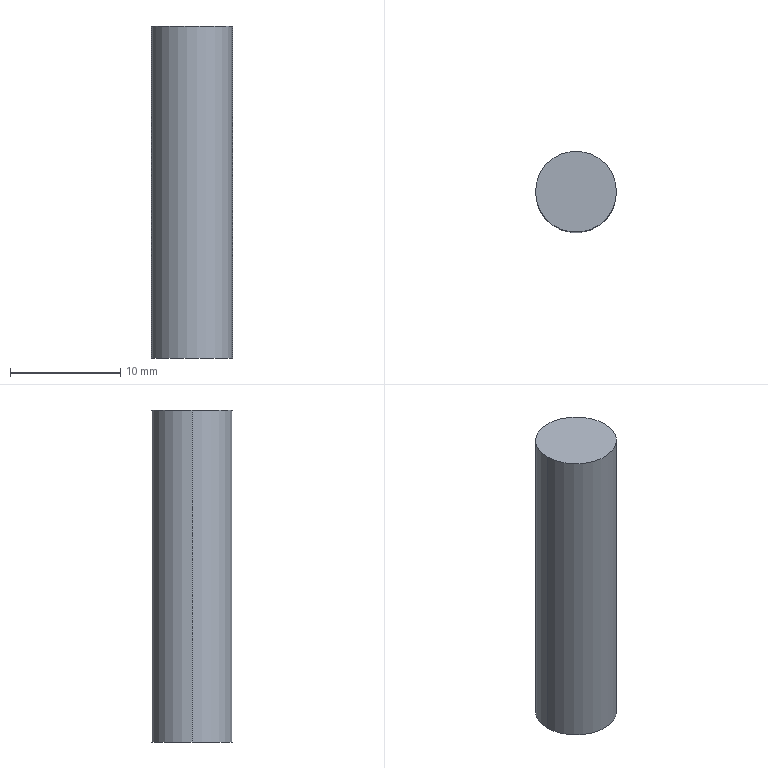Part | SolidWorks | features Extrusion 1 | 1 solid | 4 faces | box 7.349 x 7.349 x 30.108 mm | volume 1277 mm3 | cylinder 2 | plane 2 | commonest cylinder face diameters 7.349 x2
STEP:
#1=CARTESIAN_POINT('',(-23.514,-16.288,-30.108));
#2=VERTEX_POINT('',#1);
#3=CARTESIAN_POINT('',(-30.863,-16.288,-30.108));
#4=VERTEX_POINT('',#3);
#5=CARTESIAN_POINT('',(-27.189,-16.288,-30.108));
#6=DIRECTION('',(0.,0.,1.));
#7=DIRECTION('',(-1.,0.,0.));
#8=AXIS2_PLACEMENT_3D('',#5,#6,#7);
#9=CIRCLE('',#8,3.675);
#10=EDGE_CURVE('',#2,#4,#9,.T.);
#11=ORIENTED_EDGE('',*,*,#10,.T.);
#12=CARTESIAN_POINT('',(-30.863,-16.288,0.));
#13=VERTEX_POINT('',#12);
#14=CARTESIAN_POINT('',(-30.863,-16.288,-40.501));
#15=DIRECTION('',(0.,0.,1.));
#16=VECTOR('',#15,1000.);
#17=LINE('',#14,#16);
#18=EDGE_CURVE('',#4,#13,#17,.T.);
#19=ORIENTED_EDGE('',*,*,#18,.T.);
#20=CARTESIAN_POINT('',(-23.514,-16.288,0.));
#21=VERTEX_POINT('',#20);
#22=CARTESIAN_POINT('',(-27.189,-16.288,0.));
#23=DIRECTION('',(0.,0.,1.));
#24=DIRECTION('',(1.,0.,0.));
#25=AXIS2_PLACEMENT_3D('',#22,#23,#24);
#26=CIRCLE('',#25,3.675);
#27=EDGE_CURVE('',#21,#13,#26,.T.);
#28=ORIENTED_EDGE('',*,*,#27,.F.);
#29=CARTESIAN_POINT('',(-23.514,-16.288,-40.501));
#30=DIRECTION('',(0.,0.,1.));
#31=VECTOR('',#30,1000.);
#32=LINE('',#29,#31);
#33=EDGE_CURVE('',#2,#21,#32,.T.);
#34=ORIENTED_EDGE('',*,*,#33,.F.);
#35=EDGE_LOOP('',(#11,#19,#28,#34));
#36=FACE_OUTER_BOUND('',#35,.T.);
#37=CARTESIAN_POINT('',(-27.189,-16.288,-40.501));
#38=DIRECTION('',(0.,0.,1.));
#39=DIRECTION('',(1.,0.,0.));
#40=AXIS2_PLACEMENT_3D('',#37,#38,#39);
#41=CYLINDRICAL_SURFACE('',#40,3.675);
#42=ADVANCED_FACE('',(#36),#41,.T.);
#43=ORIENTED_EDGE('',*,*,#10,.F.);
#44=CARTESIAN_POINT('',(-27.189,-16.288,-30.108));
#45=DIRECTION('',(0.,0.,1.));
#46=DIRECTION('',(-1.,0.,0.));
#47=AXIS2_PLACEMENT_3D('',#44,#45,#46);
#48=CIRCLE('',#47,3.675);
#49=EDGE_CURVE('',#4,#2,#48,.T.);
#50=ORIENTED_EDGE('',*,*,#49,.F.);
#51=EDGE_LOOP('',(#43,#50));
#52=FACE_OUTER_BOUND('',#51,.T.);
#53=CARTESIAN_POINT('',(-54.131,0.,-30.108));
#54=DIRECTION('',(0.,0.,-1.));
#55=DIRECTION('',(-1.,0.,0.));
#56=AXIS2_PLACEMENT_3D('',#53,#54,#55);
#57=PLANE('',#56);
#58=ADVANCED_FACE('',(#52),#57,.T.);
#59=ORIENTED_EDGE('',*,*,#27,.T.);
#60=CARTESIAN_POINT('',(-27.189,-16.288,0.));
#61=DIRECTION('',(0.,0.,1.));
#62=DIRECTION('',(1.,0.,0.));
#63=AXIS2_PLACEMENT_3D('',#60,#61,#62);
#64=CIRCLE('',#63,3.675);
#65=EDGE_CURVE('',#13,#21,#64,.T.);
#66=ORIENTED_EDGE('',*,*,#65,.T.);
#67=EDGE_LOOP('',(#59,#66));
#68=FACE_OUTER_BOUND('',#67,.T.);
#69=CARTESIAN_POINT('',(-27.189,-16.288,0.));
#70=DIRECTION('',(0.,0.,1.));
#71=DIRECTION('',(1.,0.,0.));
#72=AXIS2_PLACEMENT_3D('',#69,#70,#71);
#73=PLANE('',#72);
#74=ADVANCED_FACE('',(#68),#73,.T.);
#75=ORIENTED_EDGE('',*,*,#18,.F.);
#76=ORIENTED_EDGE('',*,*,#49,.T.);
#77=ORIENTED_EDGE('',*,*,#33,.T.);
#78=ORIENTED_EDGE('',*,*,#65,.F.);
#79=EDGE_LOOP('',(#75,#76,#77,#78));
#80=FACE_OUTER_BOUND('',#79,.T.);
#81=CARTESIAN_POINT('',(-27.189,-16.288,-40.501));
#82=DIRECTION('',(0.,0.,1.));
#83=DIRECTION('',(1.,0.,0.));
#84=AXIS2_PLACEMENT_3D('',#81,#82,#83);
#85=CYLINDRICAL_SURFACE('',#84,3.675);
#86=ADVANCED_FACE('',(#80),#85,.T.);
#87=CLOSED_SHELL('',(#42,#58,#74,#86));
#88=MANIFOLD_SOLID_BREP('',#87);
#89=CARTESIAN_POINT('',(0.,0.,0.));
#90=DIRECTION('',(0.,0.,1.));
#91=DIRECTION('',(1.,0.,0.));
#92=AXIS2_PLACEMENT_3D('',#89,#90,#91);
#93=(LENGTH_UNIT()NAMED_UNIT(*)SI_UNIT(.MILLI.,.METRE.));
#94=UNCERTAINTY_MEASURE_WITH_UNIT(LENGTH_MEASURE(0.00001),#93,'','');
#95=(NAMED_UNIT(*)PLANE_ANGLE_UNIT()SI_UNIT($,.RADIAN.));
#96=(NAMED_UNIT(*)SI_UNIT($,.STERADIAN.)SOLID_ANGLE_UNIT());
#97=(GEOMETRIC_REPRESENTATION_CONTEXT(3)GLOBAL_UNCERTAINTY_ASSIGNED_CONTEXT((#94))GLOBAL_UNIT_ASSIGNED_CONTEXT((#93,#95,#96))REPRESENTATION_CONTEXT('',''));
#98=ADVANCED_BREP_SHAPE_REPRESENTATION('',(#88,#92),#97);